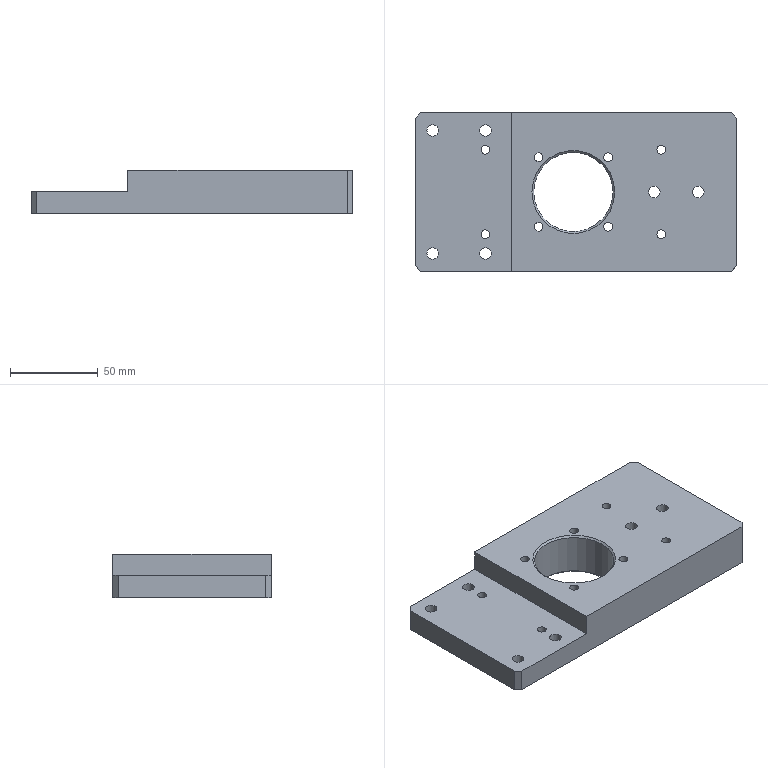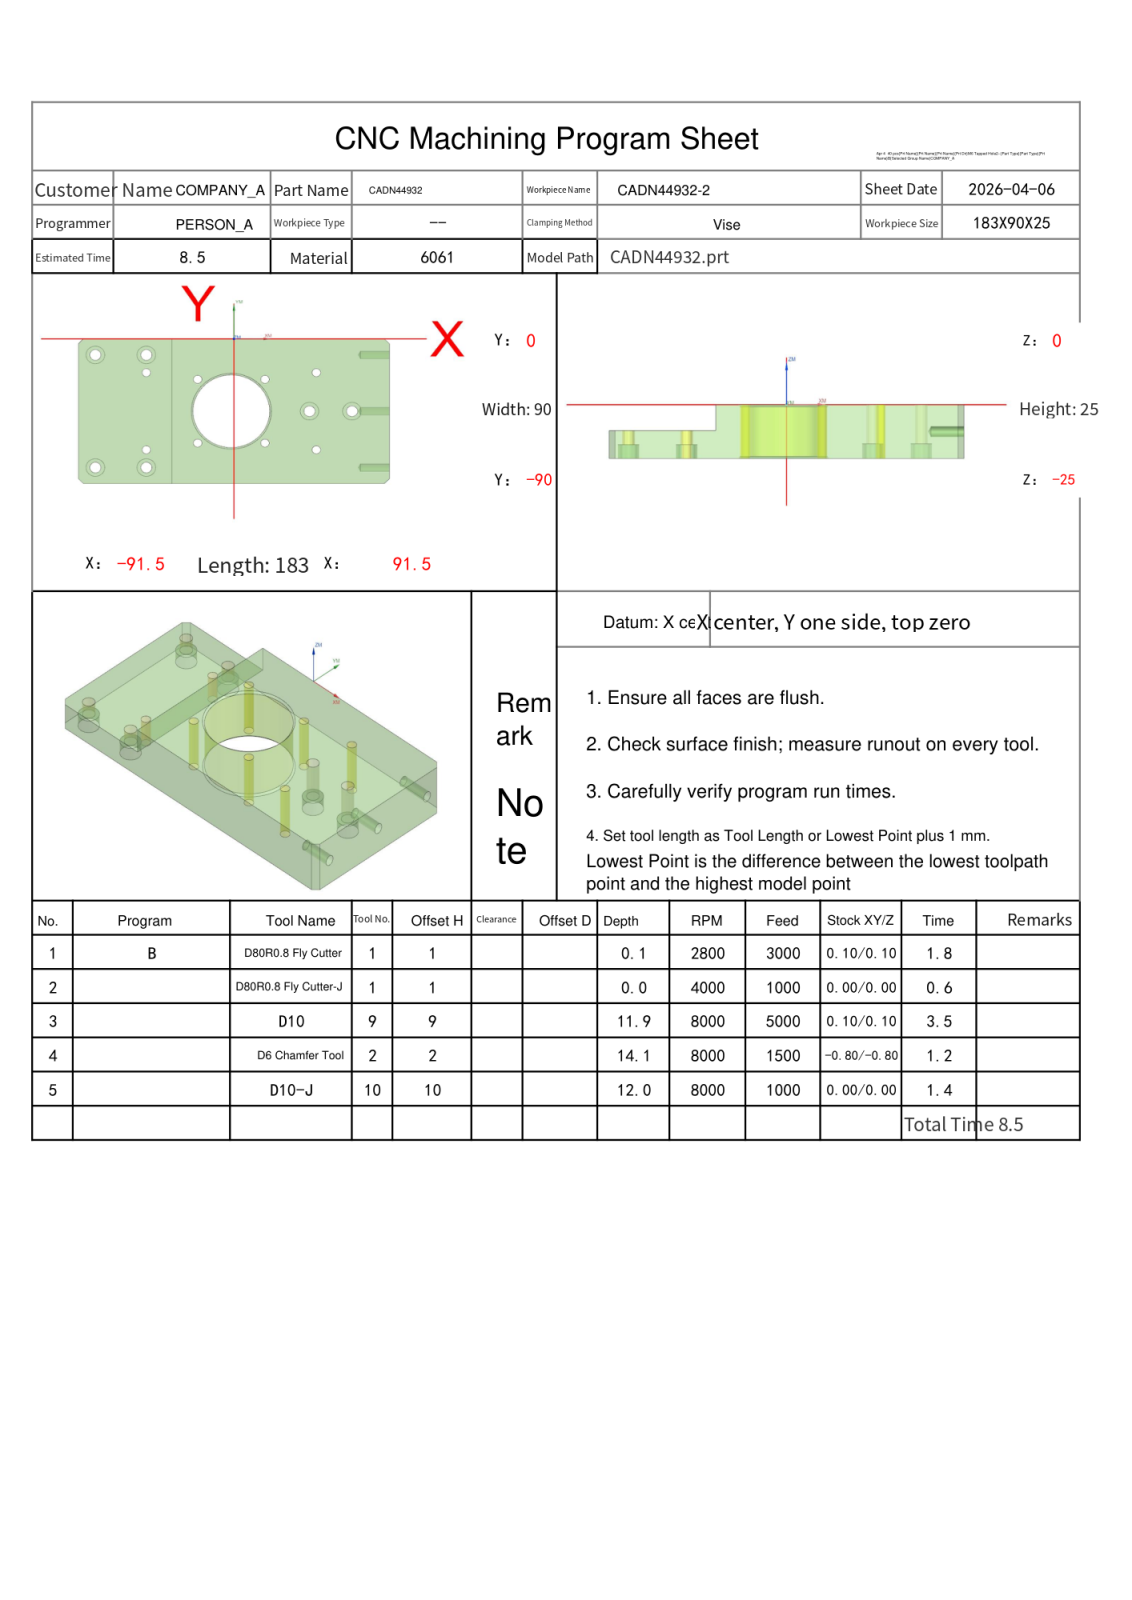NC program | NX | posted by the shop | part box 183 x 90 x 25 mm
Whole program:
%
O0001
(Machine time: 9.36 MIN)
(===Total Tool:4===)
(T1=D80R0.8 Fly Cutter D=80.  R=0.8  D-  H01 Z=0.    )
(T9=D10     D=10.  R=0.   D-  H09 Z=-11.9 )
(T2=D6 Chamfer Tool   D=6.   R=0.   D-  H02 Z=-14.1 )
(T10=D10-J  D=10.  R=0.   D10 H10 Z=-12.  )
G80 G90 G17 G49 G40
G91 G28 Z0
M01
N1 T01 M06
(D80R0.8 Fly Cutter  D=80. R=0.8 H=01 ce=0.10 di=0.10)
G00 G90 G54 X-143.597 Y-23.903 M03 S2800
G43 H01 Z20.
M08
Z6.011
G01 Z4.011 F3000.
X-131.597
X124.397
G02 X131.597 Y-31.103 I0.0 J-7.2
G01 Y-50.737
G02 X123.597 Y-58.737 I-8. J0.0
G01 X-131.597
X-143.597
Z6.011
G00 Y-23.903
Z5.522
G01 Z3.522
X-131.597
X124.397
G02 X131.597 Y-31.103 I0.0 J-7.2
G01 Y-50.737
G02 X123.597 Y-58.737 I-8. J0.0
G01 X-131.597
X-143.597
Z5.522
G00 Y-23.903
Z5.033
G01 Z3.033
X-131.597
X124.397
G02 X131.597 Y-31.103 I0.0 J-7.2
G01 Y-50.737
G02 X123.597 Y-58.737 I-8. J0.0
G01 X-131.597
X-143.597
Z5.033
G00 Y-23.903
Z4.544
G01 Z2.544
X-131.597
X124.397
G02 X131.597 Y-31.103 I0.0 J-7.2
G01 Y-50.737
G02 X123.597 Y-58.737 I-8. J0.0
G01 X-131.597
X-143.597
Z4.544
G00 Y-23.903
Z4.056
G01 Z2.056
X-131.597
X124.397
G02 X131.597 Y-31.103 I0.0 J-7.2
G01 Y-50.737
G02 X123.597 Y-58.737 I-8. J0.0
G01 X-131.597
X-143.597
Z4.056
G00 Y-23.903
Z3.567
G01 Z1.567
X-131.597
X124.397
G02 X131.597 Y-31.103 I0.0 J-7.2
G01 Y-50.737
G02 X123.597 Y-58.737 I-8. J0.0
G01 X-131.597
X-143.597
Z3.567
G00 Y-23.903
Z3.078
G01 Z1.078
X-131.597
X124.397
G02 X131.597 Y-31.103 I0.0 J-7.2
G01 Y-50.737
G02 X123.597 Y-58.737 I-8. J0.0
G01 X-131.597
X-143.597
Z3.078
G00 Y-23.903
Z2.589
G01 Z.589
X-131.597
X124.397
G02 X131.597 Y-31.103 I0.0 J-7.2
G01 Y-50.737
G02 X123.597 Y-58.737 I-8. J0.0
G01 X-131.597
X-143.597
Z2.589
G00 Y-23.903
Z2.1
G01 Z.1
X-131.597
X124.397
G02 X131.597 Y-31.103 I0.0 J-7.2
G01 Y-50.737
G02 X123.597 Y-58.737 I-8. J0.0
G01 X-131.597
X-143.597
Z2.1
G00 Z20.
G91 G28 Z0.0
M05
M09
G91 G28 Z0.0
M01
N2 T01 M06
(D80R0.8 Fly Cutter-J  D=80. R=0.8 H=01 ce=0.00 di=0.00)
G00 G90 G54 X-143.499 Y-24.001 M03 S4000
G43 H01 Z20.
M08
Z2.
G01 Z0.0 F1000.
X-131.499
X124.299
G02 X131.499 Y-31.201 I0.0 J-7.2
G01 Y-50.639
G02 X123.499 Y-58.639 I-8. J0.0
G01 X-131.499
X-143.499
Z2.
G00 Z20.
G91 G28 Z0.0
M05
M09
G91 G28 Z0.0
M01
N3 T09 M06
(D10  D=10. R=0. H=09 ce=0.10 di=0.10)
G00 G90 G54 X-94.1 Y5.714 M03 S8000
G43 H09 Z14.5
M08
Z.905
G01 Z-.595 F5000.
Y1.33
Y-90.916
G03 X-93.808 Y-91.622 I1. J.001
G01 X-90.822 Y-94.607
G03 X-90.116 Y-94.9 I.707 J.707
G01 X-87.599
G03 X-86.6 Y-93.901 I-.001 J1.
G01 Y3.901
G02 X-85.601 Y4.9 I1. J-.001
G01 X-80.099
G02 X-79.1 Y3.901 I-.001 J-1.
G01 Y-93.901
G03 X-78.101 Y-94.9 I1. J.001
G01 X-72.599
G03 X-71.6 Y-93.901 I-.001 J1.
G01 Y3.901
G02 X-70.601 Y4.9 I1. J-.001
G01 X-65.099
G02 X-64.1 Y3.901 I-.001 J-1.
G01 Y-93.901
G03 X-63.101 Y-94.9 I1. J.001
G01 X-57.599
G03 X-56.6 Y-93.901 I-.001 J1.
G01 Y3.901
G02 X-55.601 Y4.9 I1. J-.001
G01 X-50.099
G02 X-49.1 Y3.901 I-.001 J-1.
G01 Y-94.044
G03 X-48.255 Y-95.032 I1. J.001
G01 X-42.754 Y-95.888
X-42.6 Y-95.9
G03 X-41.6 Y-94.9 I0.0 J1.
G01 Y4.9
Y8.1
Z.905
G00 X-94.1 Y5.714
Z.31
G01 Z-1.19
Y1.33
Y-90.916
G03 X-93.808 Y-91.622 I1. J.001
G01 X-90.822 Y-94.607
G03 X-90.116 Y-94.9 I.707 J.707
G01 X-87.599
G03 X-86.6 Y-93.901 I-.001 J1.
G01 Y3.901
G02 X-85.601 Y4.9 I1. J-.001
G01 X-80.099
G02 X-79.1 Y3.901 I-.001 J-1.
G01 Y-93.901
G03 X-78.101 Y-94.9 I1. J.001
G01 X-72.599
G03 X-71.6 Y-93.901 I-.001 J1.
G01 Y3.901
G02 X-70.601 Y4.9 I1. J-.001
G01 X-65.099
G02 X-64.1 Y3.901 I-.001 J-1.
G01 Y-93.901
G03 X-63.101 Y-94.9 I1. J.001
G01 X-57.599
G03 X-56.6 Y-93.901 I-.001 J1.
G01 Y3.901
G02 X-55.601 Y4.9 I1. J-.001
G01 X-50.099
G02 X-49.1 Y3.901 I-.001 J-1.
G01 Y-94.044
G03 X-48.255 Y-95.032 I1. J.001
G01 X-42.754 Y-95.888
X-42.6 Y-95.9
G03 X-41.6 Y-94.9 I0.0 J1.
G01 Y4.9
Y8.1
Z.31
G00 X-94.1 Y5.714
Z-.285
G01 Z-1.785
Y1.33
Y-90.916
G03 X-93.808 Y-91.622 I1. J.001
G01 X-90.822 Y-94.607
G03 X-90.116 Y-94.9 I.707 J.707
G01 X-87.599
G03 X-86.6 Y-93.901 I-.001 J1.
G01 Y3.901
G02 X-85.601 Y4.9 I1. J-.001
G01 X-80.099
G02 X-79.1 Y3.901 I-.001 J-1.
G01 Y-93.901
G03 X-78.101 Y-94.9 I1. J.001
G01 X-72.599
G03 X-71.6 Y-93.901 I-.001 J1.
G01 Y3.901
G02 X-70.601 Y4.9 I1. J-.001
G01 X-65.099
G02 X-64.1 Y3.901 I-.001 J-1.
G01 Y-93.901
G03 X-63.101 Y-94.9 I1. J.001
G01 X-57.599
G03 X-56.6 Y-93.901 I-.001 J1.
G01 Y3.901
G02 X-55.601 Y4.9 I1. J-.001
G01 X-50.099
G02 X-49.1 Y3.901 I-.001 J-1.
G01 Y-94.044
G03 X-48.255 Y-95.032 I1. J.001
G01 X-42.754 Y-95.888
X-42.6 Y-95.9
G03 X-41.6 Y-94.9 I0.0 J1.
G01 Y4.9
Y8.1
Z-.285
G00 X-94.1 Y5.714
Z-.88
G01 Z-2.38
Y1.33
Y-90.916
G03 X-93.808 Y-91.622 I1. J.001
G01 X-90.822 Y-94.607
G03 X-90.116 Y-94.9 I.707 J.707
G01 X-87.599
G03 X-86.6 Y-93.901 I-.001 J1.
G01 Y3.901
G02 X-85.601 Y4.9 I1. J-.001
G01 X-80.099
G02 X-79.1 Y3.901 I-.001 J-1.
G01 Y-93.901
G03 X-78.101 Y-94.9 I1. J.001
G01 X-72.599
G03 X-71.6 Y-93.901 I-.001 J1.
G01 Y3.901
G02 X-70.601 Y4.9 I1. J-.001
G01 X-65.099
G02 X-64.1 Y3.901 I-.001 J-1.
G01 Y-93.901
G03 X-63.101 Y-94.9 I1. J.001
G01 X-57.599
G03 X-56.6 Y-93.901 I-.001 J1.
G01 Y3.901
G02 X-55.601 Y4.9 I1. J-.001
G01 X-50.099
G02 X-49.1 Y3.901 I-.001 J-1.
G01 Y-94.044
G03 X-48.255 Y-95.032 I1. J.001
G01 X-42.754 Y-95.888
X-42.6 Y-95.9
G03 X-41.6 Y-94.9 I0.0 J1.
G01 Y4.9
Y8.1
Z-.88
G00 X-94.1 Y5.714
Z-1.475
G01 Z-2.975
Y1.33
Y-90.916
G03 X-93.808 Y-91.622 I1. J.001
G01 X-90.822 Y-94.607
G03 X-90.116 Y-94.9 I.707 J.707
G01 X-87.599
G03 X-86.6 Y-93.901 I-.001 J1.
G01 Y3.901
G02 X-85.601 Y4.9 I1. J-.001
G01 X-80.099
G02 X-79.1 Y3.901 I-.001 J-1.
G01 Y-93.901
G03 X-78.101 Y-94.9 I1. J.001
G01 X-72.599
G03 X-71.6 Y-93.901 I-.001 J1.
G01 Y3.901
G02 X-70.601 Y4.9 I1. J-.001
G01 X-65.099
G02 X-64.1 Y3.901 I-.001 J-1.
G01 Y-93.901
G03 X-63.101 Y-94.9 I1. J.001
G01 X-57.599
G03 X-56.6 Y-93.901 I-.001 J1.
G01 Y3.901
G02 X-55.601 Y4.9 I1. J-.001
G01 X-50.099
G02 X-49.1 Y3.901 I-.001 J-1.
G01 Y-94.044
G03 X-48.255 Y-95.032 I1. J.001
G01 X-42.754 Y-95.888
X-42.6 Y-95.9
G03 X-41.6 Y-94.9 I0.0 J1.
G01 Y4.9
Y8.1
Z-1.475
G00 X-94.1 Y5.714
Z-2.07
G01 Z-3.57
Y1.33
Y-90.916
G03 X-93.808 Y-91.622 I1. J.001
G01 X-90.822 Y-94.607
G03 X-90.116 Y-94.9 I.707 J.707
G01 X-87.599
G03 X-86.6 Y-93.901 I-.001 J1.
G01 Y3.901
G02 X-85.601 Y4.9 I1. J-.001
G01 X-80.099
G02 X-79.1 Y3.901 I-.001 J-1.
G01 Y-93.901
G03 X-78.101 Y-94.9 I1. J.001
G01 X-72.599
G03 X-71.6 Y-93.901 I-.001 J1.
G01 Y3.901
G02 X-70.601 Y4.9 I1. J-.001
G01 X-65.099
G02 X-64.1 Y3.901 I-.001 J-1.
G01 Y-93.901
G03 X-63.101 Y-94.9 I1. J.001
G01 X-57.599
G03 X-56.6 Y-93.901 I-.001 J1.
G01 Y3.901
G02 X-55.601 Y4.9 I1. J-.001
G01 X-50.099
G02 X-49.1 Y3.901 I-.001 J-1.
G01 Y-94.044
G03 X-48.255 Y-95.032 I1. J.001
G01 X-42.754 Y-95.888
X-42.6 Y-95.9
G03 X-41.6 Y-94.9 I0.0 J1.
G01 Y4.9
Y8.1
Z-2.07
G00 X-94.1 Y5.714
Z-2.665
G01 Z-4.165
Y1.33
Y-90.916
G03 X-93.808 Y-91.622 I1. J.001
G01 X-90.822 Y-94.607
G03 X-90.116 Y-94.9 I.707 J.707
G01 X-87.599
G03 X-86.6 Y-93.901 I-.001 J1.
G01 Y3.901
G02 X-85.601 Y4.9 I1. J-.001
G01 X-80.099
G02 X-79.1 Y3.901 I-.001 J-1.
G01 Y-93.901
G03 X-78.101 Y-94.9 I1. J.001
G01 X-72.599
G03 X-71.6 Y-93.901 I-.001 J1.
G01 Y3.901
G02 X-70.601 Y4.9 I1. J-.001
G01 X-65.099
G02 X-64.1 Y3.901 I-.001 J-1.
G01 Y-93.901
G03 X-63.101 Y-94.9 I1. J.001
G01 X-57.599
G03 X-56.6 Y-93.901 I-.001 J1.
G01 Y3.901
G02 X-55.601 Y4.9 I1. J-.001
G01 X-50.099
G02 X-49.1 Y3.901 I-.001 J-1.
G01 Y-94.044
G03 X-48.255 Y-95.032 I1. J.001
G01 X-42.754 Y-95.888
X-42.6 Y-95.9
G03 X-41.6 Y-94.9 I0.0 J1.
G01 Y4.9
Y8.1
Z-2.665
G00 X-94.1 Y5.714
Z-3.26
G01 Z-4.76
Y1.33
Y-90.916
G03 X-93.808 Y-91.622 I1. J.001
G01 X-90.822 Y-94.607
G03 X-90.116 Y-94.9 I.707 J.707
G01 X-87.599
G03 X-86.6 Y-93.901 I-.001 J1.
G01 Y3.901
G02 X-85.601 Y4.9 I1. J-.001
G01 X-80.099
G02 X-79.1 Y3.901 I-.001 J-1.
G01 Y-93.901
G03 X-78.101 Y-94.9 I1. J.001
G01 X-72.599
G03 X-71.6 Y-93.901 I-.001 J1.
G01 Y3.901
G02 X-70.601 Y4.9 I1. J-.001
G01 X-65.099
G02 X-64.1 Y3.901 I-.001 J-1.
G01 Y-93.901
G03 X-63.101 Y-94.9 I1. J.001
G01 X-57.599
G03 X-56.6 Y-93.901 I-.001 J1.
G01 Y3.901
G02 X-55.601 Y4.9 I1. J-.001
G01 X-50.099
G02 X-49.1 Y3.901 I-.001 J-1.
G01 Y-94.044
G03 X-48.255 Y-95.032 I1. J.001
G01 X-42.754 Y-95.888
X-42.6 Y-95.9
G03 X-41.6 Y-94.9 I0.0 J1.
G01 Y4.9
Y8.1
Z-3.26
G00 X-94.1 Y5.714
Z-3.855
G01 Z-5.355
Y1.33
Y-90.916
G03 X-93.808 Y-91.622 I1. J.001
G01 X-90.822 Y-94.607
G03 X-90.116 Y-94.9 I.707 J.707
G01 X-87.599
G03 X-86.6 Y-93.901 I-.001 J1.
G01 Y3.901
G02 X-85.601 Y4.9 I1. J-.001
G01 X-80.099
G02 X-79.1 Y3.901 I-.001 J-1.
G01 Y-93.901
G03 X-78.101 Y-94.9 I1. J.001
G01 X-72.599
G03 X-71.6 Y-93.901 I-.001 J1.
G01 Y3.901
G02 X-70.601 Y4.9 I1. J-.001
G01 X-65.099
G02 X-64.1 Y3.901 I-.001 J-1.
G01 Y-93.901
G03 X-63.101 Y-94.9 I1. J.001
G01 X-57.599
G03 X-56.6 Y-93.901 I-.001 J1.
G01 Y3.901
G02 X-55.601 Y4.9 I1. J-.001
G01 X-50.099
G02 X-49.1 Y3.901 I-.001 J-1.
G01 Y-94.044
G03 X-48.255 Y-95.032 I1. J.001
G01 X-42.754 Y-95.888
X-42.6 Y-95.9
G03 X-41.6 Y-94.9 I0.0 J1.
G01 Y4.9
Y8.1
Z-3.855
G00 X-94.1 Y5.714
Z-4.45
G01 Z-5.95
Y1.33
Y-90.916
G03 X-93.808 Y-91.622 I1. J.001
G01 X-90.822 Y-94.607
G03 X-90.116 Y-94.9 I.707 J.707
G01 X-87.599
G03 X-86.6 Y-93.901 I-.001 J1.
G01 Y3.901
G02 X-85.601 Y4.9 I1. J-.001
G01 X-80.099
G02 X-79.1 Y3.901 I-.001 J-1.
G01 Y-93.901
G03 X-78.101 Y-94.9 I1. J.001
G01 X-72.599
G03 X-71.6 Y-93.901 I-.001 J1.
G01 Y3.901
G02 X-70.601 Y4.9 I1. J-.001
G01 X-65.099
G02 X-64.1 Y3.901 I-.001 J-1.
G01 Y-93.901
G03 X-63.101 Y-94.9 I1. J.001
G01 X-57.599
G03 X-56.6 Y-93.901 I-.001 J1.
G01 Y3.901
G02 X-55.601 Y4.9 I1. J-.001
G01 X-50.099
G02 X-49.1 Y3.901 I-.001 J-1.
G01 Y-94.044
G03 X-48.255 Y-95.032 I1. J.001
G01 X-42.754 Y-95.888
X-42.6 Y-95.9
G03 X-41.6 Y-94.9 I0.0 J1.
G01 Y4.9
Y8.1
Z-4.45
G00 X-94.1 Y5.714
Z-5.045
G01 Z-6.545
Y1.33
Y-90.916
G03 X-93.808 Y-91.622 I1. J.001
G01 X-90.822 Y-94.607
G03 X-90.116 Y-94.9 I.707 J.707
G01 X-87.599
G03 X-86.6 Y-93.901 I-.001 J1.
G01 Y3.901
G02 X-85.601 Y4.9 I1. J-.001
G01 X-80.099
G02 X-79.1 Y3.901 I-.001 J-1.
G01 Y-93.901
G03 X-78.101 Y-94.9 I1. J.001
G01 X-72.599
G03 X-71.6 Y-93.901 I-.001 J1.
G01 Y3.901
G02 X-70.601 Y4.9 I1. J-.001
G01 X-65.099
G02 X-64.1 Y3.901 I-.001 J-1.
G01 Y-93.901
G03 X-63.101 Y-94.9 I1. J.001
G01 X-57.599
G03 X-56.6 Y-93.901 I-.001 J1.
G01 Y3.901
G02 X-55.601 Y4.9 I1. J-.001
G01 X-50.099
G02 X-49.1 Y3.901 I-.001 J-1.
G01 Y-94.044
G03 X-48.255 Y-95.032 I1. J.001
G01 X-42.754 Y-95.888
X-42.6 Y-95.9
G03 X-41.6 Y-94.9 I0.0 J1.
G01 Y4.9
Y8.1
Z-5.045
G00 X-94.1 Y5.714
Z-5.64
G01 Z-7.14
Y1.33
Y-90.916
G03 X-93.808 Y-91.622 I1. J.001
G01 X-90.822 Y-94.607
G03 X-90.116 Y-94.9 I.707 J.707
G01 X-87.599
G03 X-86.6 Y-93.901 I-.001 J1.
G01 Y3.901
G02 X-85.601 Y4.9 I1. J-.001
G01 X-80.099
G02 X-79.1 Y3.901 I-.001 J-1.
G01 Y-93.901
G03 X-78.101 Y-94.9 I1. J.001
G01 X-72.599
G03 X-71.6 Y-93.901 I-.001 J1.
G01 Y3.901
G02 X-70.601 Y4.9 I1. J-.001
G01 X-65.099
G02 X-64.1 Y3.901 I-.001 J-1.
G01 Y-93.901
G03 X-63.101 Y-94.9 I1. J.001
G01 X-57.599
G03 X-56.6 Y-93.901 I-.001 J1.
G01 Y3.901
G02 X-55.601 Y4.9 I1. J-.001
G01 X-50.099
G02 X-49.1 Y3.901 I-.001 J-1.
G01 Y-94.044
G03 X-48.255 Y-95.032 I1. J.001
G01 X-42.754 Y-95.888
X-42.6 Y-95.9
G03 X-41.6 Y-94.9 I0.0 J1.
G01 Y4.9
Y8.1
Z-5.64
G00 X-94.1 Y5.714
Z-6.235
G01 Z-7.735
Y1.33
Y-90.916
G03 X-93.808 Y-91.622 I1. J.001
G01 X-90.822 Y-94.607
G03 X-90.116 Y-94.9 I.707 J.707
G01 X-87.599
G03 X-86.6 Y-93.901 I-.001 J1.
G01 Y3.901
G02 X-85.601 Y4.9 I1. J-.001
G01 X-80.099
G02 X-79.1 Y3.901 I-.001 J-1.
G01 Y-93.901
G03 X-78.101 Y-94.9 I1. J.001
G01 X-72.599
G03 X-71.6 Y-93.901 I-.001 J1.
G01 Y3.901
G02 X-70.601 Y4.9 I1. J-.001
G01 X-65.099
G02 X-64.1 Y3.901 I-.001 J-1.
G01 Y-93.901
G03 X-63.101 Y-94.9 I1. J.001
G01 X-57.599
G03 X-56.6 Y-93.901 I-.001 J1.
G01 Y3.901
G02 X-55.601 Y4.9 I1. J-.001
G01 X-50.099
G02 X-49.1 Y3.901 I-.001 J-1.
G01 Y-94.044
G03 X-48.255 Y-95.032 I1. J.001
G01 X-42.754 Y-95.888
X-42.6 Y-95.9
G03 X-41.6 Y-94.9 I0.0 J1.
G01 Y4.9
Y8.1
Z-6.235
G00 X-94.1 Y5.714
Z-6.83
G01 Z-8.33
Y1.33
Y-90.916
G03 X-93.808 Y-91.622 I1. J.001
G01 X-90.822 Y-94.607
G03 X-90.116 Y-94.9 I.707 J.707
G01 X-87.599
G03 X-86.6 Y-93.901 I-.001 J1.
G01 Y3.901
G02 X-85.601 Y4.9 I1. J-.001
G01 X-80.099
G02 X-79.1 Y3.901 I-.001 J-1.
G01 Y-93.901
G03 X-78.101 Y-94.9 I1. J.001
G01 X-72.599
G03 X-71.6 Y-93.901 I-.001 J1.
G01 Y3.901
G02 X-70.601 Y4.9 I1. J-.001
G01 X-65.099
G02 X-64.1 Y3.901 I-.001 J-1.
G01 Y-93.901
G03 X-63.101 Y-94.9 I1. J.001
G01 X-57.599
G03 X-56.6 Y-93.901 I-.001 J1.
G01 Y3.901
G02 X-55.601 Y4.9 I1. J-.001
G01 X-50.099
G02 X-49.1 Y3.901 I-.001 J-1.
G01 Y-94.044
G03 X-48.255 Y-95.032 I1. J.001
G01 X-42.754 Y-95.888
X-42.6 Y-95.9
G03 X-41.6 Y-94.9 I0.0 J1.
G01 Y4.9
Y8.1
Z-6.83
G00 X-94.1 Y5.714
Z-7.425
G01 Z-8.925
Y1.33
Y-90.916
G03 X-93.808 Y-91.622 I1. J.001
G01 X-90.822 Y-94.607
G03 X-90.116 Y-94.9 I.707 J.707
G01 X-87.599
G03 X-86.6 Y-93.901 I-.001 J1.
G01 Y3.901
G02 X-85.601 Y4.9 I1. J-.001
G01 X-80.099
G02 X-79.1 Y3.901 I-.001 J-1.
G01 Y-93.901
G03 X-78.101 Y-94.9 I1. J.001
G01 X-72.599
G03 X-71.6 Y-93.901 I-.001 J1.
G01 Y3.901
G02 X-70.601 Y4.9 I1. J-.001
G01 X-65.099
G02 X-64.1 Y3.901 I-.001 J-1.
G01 Y-93.901
G03 X-63.101 Y-94.9 I1. J.001
G01 X-57.599
G03 X-56.6 Y-93.901 I-.001 J1.
G01 Y3.901
G02 X-55.601 Y4.9 I1. J-.001
G01 X-50.099
G02 X-49.1 Y3.901 I-.001 J-1.
G01 Y-94.044
G03 X-48.255 Y-95.032 I1. J.001
G01 X-42.754 Y-95.888
X-42.6 Y-95.9
G03 X-41.6 Y-94.9 I0.0 J1.
G01 Y4.9
Y8.1
Z-7.425
G00 X-94.1 Y5.714
Z-8.02
G01 Z-9.52
Y1.33
Y-90.916
G03 X-93.808 Y-91.622 I1. J.001
G01 X-90.822 Y-94.607
G03 X-90.116 Y-94.9 I.707 J.707
G01 X-87.599
G03 X-86.6 Y-93.901 I-.001 J1.
G01 Y3.901
G02 X-85.601 Y4.9 I1. J-.001
G01 X-80.099
G02 X-79.1 Y3.901 I-.001 J-1.
G01 Y-93.901
G03 X-78.101 Y-94.9 I1. J.001
G01 X-72.599
G03 X-71.6 Y-93.901 I-.001 J1.
G01 Y3.901
G02 X-70.601 Y4.9 I1. J-.001
G01 X-65.099
G02 X-64.1 Y3.901 I-.001 J-1.
G01 Y-93.901
G03 X-63.101 Y-94.9 I1. J.001
G01 X-57.599
G03 X-56.6 Y-93.901 I-.001 J1.
G01 Y3.901
G02 X-55.601 Y4.9 I1. J-.001
G01 X-50.099
G02 X-49.1 Y3.901 I-.001 J-1.
G01 Y-94.044
G03 X-48.255 Y-95.032 I1. J.001
G01 X-42.754 Y-95.888
X-42.6 Y-95.9
G03 X-41.6 Y-94.9 I0.0 J1.
G01 Y4.9
Y8.1
Z-8.02
G00 X-94.1 Y5.714
Z-8.615
G01 Z-10.115
Y1.33
Y-90.916
G03 X-93.808 Y-91.622 I1. J.001
G01 X-90.822 Y-94.607
G03 X-90.116 Y-94.9 I.707 J.707
G01 X-87.599
G03 X-86.6 Y-93.901 I-.001 J1.
G01 Y3.901
G02 X-85.601 Y4.9 I1. J-.001
G01 X-80.099
G02 X-79.1 Y3.901 I-.001 J-1.
G01 Y-93.901
G03 X-78.101 Y-94.9 I1. J.001
G01 X-72.599
G03 X-71.6 Y-93.901 I-.001 J1.
G01 Y3.901
G02 X-70.601 Y4.9 I1. J-.001
G01 X-65.099
G02 X-64.1 Y3.901 I-.001 J-1.
G01 Y-93.901
G03 X-63.101 Y-94.9 I1. J.001
G01 X-57.599
G03 X-56.6 Y-93.901 I-.001 J1.
G01 Y3.901
G02 X-55.601 Y4.9 I1. J-.001
G01 X-50.099
G02 X-49.1 Y3.901 I-.001 J-1.
G01 Y-94.044
G03 X-48.255 Y-95.032 I1. J.001
G01 X-42.754 Y-95.888
X-42.6 Y-95.9
G03 X-41.6 Y-94.9 I0.0 J1.
G01 Y4.9
Y8.1
Z-8.615
G00 X-94.1 Y5.714
Z-9.21
G01 Z-10.71
Y1.33
Y-90.916
G03 X-93.808 Y-91.622 I1. J.001
G01 X-90.822 Y-94.607
G03 X-90.116 Y-94.9 I.707 J.707
G01 X-87.599
G03 X-86.6 Y-93.901 I-.001 J1.
G01 Y3.901
G02 X-85.601 Y4.9 I1. J-.001
G01 X-80.099
G02 X-79.1 Y3.901 I-.001 J-1.
G01 Y-93.901
G03 X-78.101 Y-94.9 I1. J.001
G01 X-72.599
G03 X-71.6 Y-93.901 I-.001 J1.
G01 Y3.901
G02 X-70.601 Y4.9 I1. J-.001
G01 X-65.099
G02 X-64.1 Y3.901 I-.001 J-1.
G01 Y-93.901
G03 X-63.101 Y-94.9 I1. J.001
G01 X-57.599
G03 X-56.6 Y-93.901 I-.001 J1.
G01 Y3.901
G02 X-55.601 Y4.9 I1. J-.001
G01 X-50.099
G02 X-49.1 Y3.901 I-.001 J-1.
G01 Y-94.044
G03 X-48.255 Y-95.032 I1. J.001
G01 X-42.754 Y-95.888
X-42.6 Y-95.9
G03 X-41.6 Y-94.9 I0.0 J1.
G01 Y4.9
Y8.1
Z-9.21
G00 X-94.1 Y5.714
Z-9.805
G01 Z-11.305
Y1.33
Y-90.916
G03 X-93.808 Y-91.622 I1. J.001
G01 X-90.822 Y-94.607
G03 X-90.116 Y-94.9 I.707 J.707
G01 X-87.599
G03 X-86.6 Y-93.901 I-.001 J1.
G01 Y3.901
G02 X-85.601 Y4.9 I1. J-.001
G01 X-80.099
G02 X-79.1 Y3.901 I-.001 J-1.
G01 Y-93.901
G03 X-78.101 Y-94.9 I1. J.001
G01 X-72.599
G03 X-71.6 Y-93.901 I-.001 J1.
G01 Y3.901
G02 X-70.601 Y4.9 I1. J-.001
G01 X-65.099
G02 X-64.1 Y3.901 I-.001 J-1.
G01 Y-93.901
G03 X-63.101 Y-94.9 I1. J.001
G01 X-57.599
G03 X-56.6 Y-93.901 I-.001 J1.
G01 Y3.901
G02 X-55.601 Y4.9 I1. J-.001
G01 X-50.099
G02 X-49.1 Y3.901 I-.001 J-1.
G01 Y-94.044
G03 X-48.255 Y-95.032 I1. J.001
G01 X-42.754 Y-95.888
X-42.6 Y-95.9
G03 X-41.6 Y-94.9 I0.0 J1.
G01 Y4.9
Y8.1
Z-9.805
G00 X-94.1 Y5.714
Z-10.4
G01 Z-11.9
Y1.33
Y-90.916
G03 X-93.808 Y-91.622 I1. J.001
G01 X-90.822 Y-94.607
G03 X-90.116 Y-94.9 I.707 J.707
G01 X-87.599
G03 X-86.6 Y-93.901 I-.001 J1.
G01 Y3.901
G02 X-85.601 Y4.9 I1. J-.001
G01 X-80.099
G02 X-79.1 Y3.901 I-.001 J-1.
G01 Y-93.901
G03 X-78.101 Y-94.9 I1. J.001
G01 X-72.599
G03 X-71.6 Y-93.901 I-.001 J1.
G01 Y3.901
G02 X-70.601 Y4.9 I1. J-.001
G01 X-65.099
G02 X-64.1 Y3.901 I-.001 J-1.
G01 Y-93.901
G03 X-63.101 Y-94.9 I1. J.001
G01 X-57.599
G03 X-56.6 Y-93.901 I-.001 J1.
G01 Y3.901
G02 X-55.601 Y4.9 I1. J-.001
G01 X-50.099
G02 X-49.1 Y3.901 I-.001 J-1.
G01 Y-94.044
G03 X-48.255 Y-95.032 I1. J.001
G01 X-42.754 Y-95.888
X-42.6 Y-95.9
G03 X-41.6 Y-94.9 I0.0 J1.
G01 Y4.9
Y8.1
Z-10.4
G00 Z14.5
G91 G28 Z0.0
M05
M09
G91 G28 Z0.0
M01
N4 T02 M06
(D6 Chamfer Tool  D=6. R=0. H=02 ce=-0.30 di=0.00)
G00 G90 G54 X18.27 Y-54.309 M03 S7000
G43 H02 Z20.
M08
Z2.5
G01 X18.288 Y-54.272 Z2.485 F1500.
X18.701 Y-53.335 Z2.112
X19.069 Y-52.38 Z1.74
X19.392 Y-51.409 Z1.367
X19.669 Y-50.424 Z.995
X19.9 Y-49.426 Z.622
X20.084 Y-48.419 Z.25
X20.22 Y-47.405 Z-.123
X20.309 Y-46.385 Z-.496
X20.35 Y-45.362 Z-.868
Y-45. Z-1.
G03 X-1.5 Y-23.15 I-21.85 J0.0
X-23.35 Y-45. I0.0 J-21.85
X-1.5 Y-66.85 I21.85 J0.0
X20.35 Y-45. I0.0 J21.85
X20.344 Y-44.5 I-21.85 J0.0
G01 Z1.5
G00 Z20.
G00 G90 X48.732 Y-21.87 M03 S8000
Z20.
Z-.9
G01 Z-1.4 F600.
X48.9 Y-22.5
G03 X50.4 Y-21. I0.0 J1.5
X48.5 Y-19.1 I-1.9 J0.0
X46.6 Y-21. I0.0 J-1.9
X48.5 Y-22.9 I1.9 J0.0
X50.4 Y-21. I0.0 J1.9
X48.9 Y-19.5 I-1.5 J0.0
G01 X48.732 Y-20.13
Z-.9
G00 Z20.
X18.531 Y-26.071
Z-.9
G01 Z-1.4
X18.699 Y-26.701
G03 X20.199 Y-25.201 I0.0 J1.5
X18.299 Y-23.301 I-1.9 J0.0
X16.399 Y-25.201 I0.0 J-1.9
X18.299 Y-27.101 I1.9 J0.0
X20.199 Y-25.201 I0.0 J1.9
X18.699 Y-23.701 I-1.5 J0.0
G01 X18.531 Y-24.331
Z-.9
G00 Z20.
X-21.067 Y-26.071
Z-.9
G01 Z-1.4
X-20.899 Y-26.701
G03 X-19.399 Y-25.201 I0.0 J1.5
X-21.299 Y-23.301 I-1.9 J0.0
X-23.199 Y-25.201 I0.0 J-1.9
X-21.299 Y-27.101 I1.9 J0.0
X-19.399 Y-25.201 I0.0 J1.9
X-20.899 Y-23.701 I-1.5 J0.0
G01 X-21.067 Y-24.331
Z-.9
G00 Z20.
Y-65.669
Z-.9
G01 Z-1.4
X-20.899 Y-66.299
G03 X-19.399 Y-64.799 I0.0 J1.5
X-21.299 Y-62.899 I-1.9 J0.0
X-23.199 Y-64.799 I0.0 J-1.9
X-21.299 Y-66.699 I1.9 J0.0
X-19.399 Y-64.799 I0.0 J1.9
X-20.899 Y-63.299 I-1.5 J0.0
G01 X-21.067 Y-63.929
Z-.9
G00 Z20.
X18.531 Y-65.669
Z-.9
G01 Z-1.4
X18.699 Y-66.299
G03 X20.199 Y-64.799 I0.0 J1.5
X18.299 Y-62.899 I-1.9 J0.0
X16.399 Y-64.799 I0.0 J-1.9
X18.299 Y-66.699 I1.9 J0.0
X20.199 Y-64.799 I0.0 J1.9
X18.699 Y-63.299 I-1.5 J0.0
G01 X18.531 Y-63.929
Z-.9
G00 Z20.
X48.732 Y-69.87
Z-.9
G01 Z-1.4
X48.9 Y-70.5
G03 X50.4 Y-69. I0.0 J1.5
X48.5 Y-67.1 I-1.9 J0.0
X46.6 Y-69. I0.0 J-1.9
X48.5 Y-70.9 I1.9 J0.0
X50.4 Y-69. I0.0 J1.9
X48.9 Y-67.5 I-1.5 J0.0
G01 X48.732 Y-68.13
Z-.9
G00 Z20.
G00 G90 X-51.437 Y-69.19 M03 S8000
Z20.
Z-13.6
G01 Z-14.1 F600.
X-51.426 Y-69.224
G03 X-51.133 Y-69.253 I.293 J1.471
X-50.3 Y-69. I0.0 J1.5
X-51.5 Y-67.8 I-1.2 J0.0
X-52.7 Y-69. I0.0 J-1.2
X-51.5 Y-70.2 I1.2 J0.0
X-50.3 Y-69. I0.0 J1.2
X-51.133 Y-68.747 I-.833 J-1.247
X-51.426 Y-68.776 I0.0 J-1.5
G01 X-51.437 Y-68.81
Z-13.6
G00 Z20.
Y-21.19
Z-13.6
G01 Z-14.1
X-51.426 Y-21.224
G03 X-51.133 Y-21.253 I.293 J1.471
X-50.3 Y-21. I0.0 J1.5
X-51.5 Y-19.8 I-1.2 J0.0
X-52.7 Y-21. I0.0 J-1.2
X-51.5 Y-22.2 I1.2 J0.0
X-50.3 Y-21. I0.0 J1.2
X-51.133 Y-20.747 I-.833 J-1.247
X-51.426 Y-20.776 I0.0 J-1.5
G01 X-51.437 Y-20.81
Z-13.6
G00 Z20.
G00 G90 X25.614 Y1.227 M03 S6500
Z20.
Z.172
G01 Z-1.2 F1500.
G03 X25.9 Y1.027 I1.286 J1.532
G01 X25.946 Y.997
X26. Y1.
X88.5
X88.759 Y.966
X89. Y.866
X89.207 Y.707
X92.207 Y-2.293
X92.366 Y-2.5
X92.466 Y-2.741
X92.5 Y-3.
Y-87.
X92.466 Y-87.259
X92.366 Y-87.5
X92.207 Y-87.707
X89.207 Y-90.707
X89. Y-90.866
X88.759 Y-90.966
X88.5 Y-91.
X-36.5
G02 X-37.5 Y-90. I0.0 J1.
G01 Y0.0
G02 X-36.5 Y1. I1. J0.0
G01 X26.
X26.054 Y.997
X26.1 Y1.027
G03 X26.386 Y1.227 I-1. J1.732
G01 Z.172
G00 Z10.
X-19.984 Y-65.206
Z.284
G01 Z-1.2
G03 X-19.815 Y-64.901 I-1.658 J1.118
G01 X-19.79 Y-64.853
X-19.799 Y-64.799
G03 X-21.299 Y-63.299 I-1.5 J0.0
X-22.799 Y-64.799 I0.0 J-1.5
X-21.299 Y-66.299 I1.5 J0.0
X-19.799 Y-64.799 I0.0 J1.5
G01 X-19.79 Y-64.745
X-19.815 Y-64.697
G03 X-19.984 Y-64.392 I-1.827 J-.813
G01 Z.284
G00 Z10.
Y-25.608
Z.284
G01 Z-1.2
G03 X-19.815 Y-25.303 I-1.658 J1.118
G01 X-19.79 Y-25.255
X-19.799 Y-25.201
G03 X-21.299 Y-23.701 I-1.5 J0.0
X-22.799 Y-25.201 I0.0 J-1.5
X-21.299 Y-26.701 I1.5 J0.0
X-19.799 Y-25.201 I0.0 J1.5
G01 X-19.79 Y-25.147
X-19.815 Y-25.099
G03 X-19.984 Y-24.794 I-1.827 J-.813
G01 Z.284
G00 Z10.
X19.614 Y-25.608
Z.284
G01 Z-1.2
G03 X19.783 Y-25.303 I-1.658 J1.118
G01 X19.808 Y-25.255
X19.799 Y-25.201
G03 X18.299 Y-23.701 I-1.5 J0.0
X16.799 Y-25.201 I0.0 J-1.5
X18.299 Y-26.701 I1.5 J0.0
X19.799 Y-25.201 I0.0 J1.5
G01 X19.808 Y-25.147
X19.783 Y-25.099
G03 X19.614 Y-24.794 I-1.827 J-.813
G01 Z.284
G00 Z10.
X49.815 Y-21.407
Z.284
G01 Z-1.2
G03 X49.984 Y-21.102 I-1.658 J1.118
G01 X50.009 Y-21.054
X50. Y-21.
G03 X48.5 Y-19.5 I-1.5 J0.0
X47. Y-21. I0.0 J-1.5
X48.5 Y-22.5 I1.5 J0.0
X50. Y-21. I0.0 J1.5
G01 X50.009 Y-20.946
X49.984 Y-20.898
G03 X49.815 Y-20.593 I-1.827 J-.813
G01 Z.284
G00 Z10.
X71.608 Y-45.404
Z.253
G01 Z-1.2
G03 X71.782 Y-45.102 I-1.638 J1.147
G01 X71.808 Y-45.054
X71.8 Y-45.
G03 X69.5 Y-42.7 I-2.3 J0.0
X67.2 Y-45. I0.0 J-2.3
X69.5 Y-47.3 I2.3 J0.0
X71.8 Y-45. I0.0 J2.3
G01 X71.808 Y-44.946
X71.782 Y-44.898
G03 X71.608 Y-44.596 I-1.813 J-.845
G01 Z.253
G00 Z10.
X46.608 Y-45.404
Z.253
G01 Z-1.2
G03 X46.782 Y-45.102 I-1.638 J1.147
G01 X46.808 Y-45.054
X46.8 Y-45.
G03 X44.5 Y-42.7 I-2.3 J0.0
X42.2 Y-45. I0.0 J-2.3
X44.5 Y-47.3 I2.3 J0.0
X46.8 Y-45. I0.0 J2.3
G01 X46.808 Y-44.946
X46.782 Y-44.898
G03 X46.608 Y-44.596 I-1.813 J-.845
G01 Z.253
G00 Z10.
X49.815 Y-69.407
Z.284
G01 Z-1.2
G03 X49.984 Y-69.102 I-1.658 J1.118
G01 X50.009 Y-69.054
X50. Y-69.
G03 X48.5 Y-67.5 I-1.5 J0.0
X47. Y-69. I0.0 J-1.5
X48.5 Y-70.5 I1.5 J0.0
X50. Y-69. I0.0 J1.5
G01 X50.009 Y-68.946
X49.984 Y-68.898
G03 X49.815 Y-68.593 I-1.827 J-.813
G01 Z.284
G00 Z10.
X19.614 Y-65.206
Z.284
G01 Z-1.2
G03 X19.783 Y-64.901 I-1.658 J1.118
G01 X19.808 Y-64.853
X19.799 Y-64.799
G03 X18.299 Y-63.299 I-1.5 J0.0
X16.799 Y-64.799 I0.0 J-1.5
X18.299 Y-66.299 I1.5 J0.0
X19.799 Y-64.799 I0.0 J1.5
G01 X19.808 Y-64.745
X19.783 Y-64.697
G03 X19.614 Y-64.392 I-1.827 J-.813
G01 Z.284
G00 Z10.
X-39.507 Y-91.068
Z-1.793
G01 Z-13.2
X-39.593 Y-91.008
X-39.623 Y-91.
X-88.5
X-88.759 Y-90.966
X-89. Y-90.866
X-89.207 Y-90.707
X-92.207 Y-87.707
X-92.366 Y-87.5
X-92.466 Y-87.259
X-92.5 Y-87.
Y-3.
X-92.466 Y-2.741
X-92.366 Y-2.5
X-92.207 Y-2.293
X-89.207 Y.707
X-89. Y.866
X-88.759 Y.966
X-88.5 Y1.
X-39.623
X-39.593 Y1.008
X-39.507 Y1.068
Z-1.793
G00 Z10.
X-79.392 Y-10.404
Z-11.747
G01 Z-13.2
G03 X-79.218 Y-10.102 I-1.638 J1.147
G01 X-79.192 Y-10.054
X-79.2 Y-10.
G03 X-81.5 Y-7.7 I-2.3 J0.0
X-83.8 Y-10. I0.0 J-2.3
X-81.5 Y-12.3 I2.3 J0.0
X-79.2 Y-10. I0.0 J2.3
G01 X-79.192 Y-9.946
X-79.218 Y-9.898
G03 X-79.392 Y-9.596 I-1.813 J-.845
G01 Z-11.747
G00 Z10.
X-49.392 Y-10.404
Z-11.747
G01 Z-13.2
G03 X-49.218 Y-10.102 I-1.638 J1.147
G01 X-49.192 Y-10.054
X-49.2 Y-10.
G03 X-51.5 Y-7.7 I-2.3 J0.0
X-53.8 Y-10. I0.0 J-2.3
X-51.5 Y-12.3 I2.3 J0.0
X-49.2 Y-10. I0.0 J2.3
G01 X-49.192 Y-9.946
X-49.218 Y-9.898
G03 X-49.392 Y-9.596 I-1.813 J-.845
G01 Z-11.747
G00 Z-9.45
X-50.185 Y-21.407
Z-11.716
G01 Z-13.2
G03 X-50.016 Y-21.102 I-1.658 J1.118
G01 X-49.991 Y-21.054
X-50. Y-21.
G03 X-51.5 Y-19.5 I-1.5 J0.0
X-53. Y-21. I0.0 J-1.5
X-51.5 Y-22.5 I1.5 J0.0
X-50. Y-21. I0.0 J1.5
G01 X-49.991 Y-20.946
X-50.016 Y-20.898
G03 X-50.185 Y-20.593 I-1.827 J-.813
G01 Z-11.716
G00 Z10.
Y-69.407
Z-11.716
G01 Z-13.2
G03 X-50.016 Y-69.102 I-1.658 J1.118
G01 X-49.991 Y-69.054
X-50. Y-69.
G03 X-51.5 Y-67.5 I-1.5 J0.0
X-53. Y-69. I0.0 J-1.5
X-51.5 Y-70.5 I1.5 J0.0
X-50. Y-69. I0.0 J1.5
G01 X-49.991 Y-68.946
X-50.016 Y-68.898
G03 X-50.185 Y-68.593 I-1.827 J-.813
G01 Z-11.716
G00 Z-9.45
X-49.392 Y-80.404
Z-11.747
G01 Z-13.2
G03 X-49.218 Y-80.102 I-1.638 J1.147
G01 X-49.192 Y-80.054
X-49.2 Y-80.
G03 X-51.5 Y-77.7 I-2.3 J0.0
X-53.8 Y-80. I0.0 J-2.3
X-51.5 Y-82.3 I2.3 J0.0
X-49.2 Y-80. I0.0 J2.3
G01 X-49.192 Y-79.946
X-49.218 Y-79.898
G03 X-49.392 Y-79.596 I-1.813 J-.845
G01 Z-11.747
G00 Z10.
X-79.392 Y-80.404
Z-11.747
G01 Z-13.2
G03 X-79.218 Y-80.102 I-1.638 J1.147
G01 X-79.192 Y-80.054
X-79.2 Y-80.
G03 X-81.5 Y-77.7 I-2.3 J0.0
X-83.8 Y-80. I0.0 J-2.3
X-81.5 Y-82.3 I2.3 J0.0
X-79.2 Y-80. I0.0 J2.3
G01 X-79.192 Y-79.946
X-79.218 Y-79.898
G03 X-79.392 Y-79.596 I-1.813 J-.845
G01 Z-11.747
G00 Z20.
G00 G90 X-.3 Y-24.385 M03 S6500
Z20.
Z-.2
G01 Z-1.7 F1500.
Y-24.35
G03 X-1.5 Y-23.15 I-1.2 J0.0
X-23.35 Y-45. I0.0 J-21.85
X-1.5 Y-66.85 I21.85 J0.0
X20.35 Y-45. I0.0 J21.85
X-1.5 Y-23.15 I-21.85 J0.0
X-1.9 Y-23.154 I0.0 J-21.85
X-3.078 Y-24.353 I.022 J-1.2
G01 Y-24.375
X-3.077 Y-24.41
Z-.2
G00 Z20.
G91 G28 Z0.0
M05
M09
G91 G28 Z0.0
M01
N5 T10 M06
(D10-J  D=10. R=0. H=10 ce=0.40 di=0.00)
G00 G90 G54 X-93.562 Y-94.837 M03 S8000
G43 H10 Z14.5
M08
Z-10.5
G01 Z-12. F1000.
G03 X-92.5 Y-93.071 I-.938 J1.766
G01 Y2.658
G02 X-92.208 Y3.363 I1. J-.001
G01 X-90.864 Y4.707
G02 X-90.157 Y5. I.707 J-.707
G01 X-88.899
G02 X-87.9 Y4.001 I-.001 J-1.
G01 Y-94.1
G03 X-87. Y-95. I.9 J0.0
G01 X-84.3
G03 X-83.3 Y-94. I0.0 J1.
G01 Y4.1
G02 X-82.4 Y5. I.9 J0.0
G01 X-79.7
G02 X-78.7 Y4. I0.0 J-1.
G01 Y-94.1
G03 X-77.8 Y-95. I.9 J0.0
G01 X-75.1
G03 X-74.1 Y-94. I0.0 J1.
G01 Y4.1
G02 X-73.2 Y5. I.9 J0.0
G01 X-70.5
G02 X-69.5 Y4. I0.0 J-1.
G01 Y-94.1
G03 X-68.6 Y-95. I.9 J0.0
G01 X-65.9
G03 X-64.9 Y-94. I0.0 J1.
G01 Y4.1
G02 X-64. Y5. I.9 J0.0
G01 X-61.3
G02 X-60.3 Y4. I0.0 J-1.
G01 Y-94.1
G03 X-59.4 Y-95. I.9 J0.0
G01 X-56.7
G03 X-55.7 Y-94. I0.0 J1.
G01 Y4.1
G02 X-54.8 Y5. I.9 J0.0
G01 X-52.1
G02 X-51.1 Y4. I0.0 J-1.
G01 Y-94.1
G03 X-50.2 Y-95. I.9 J0.0
G01 X-47.5
G03 X-46.5 Y-94. I0.0 J1.
G01 Y4.1
G02 X-45.6 Y5. I.9 J0.0
G01 X-42.9
G02 X-41.9 Y4. I0.0 J-1.
G01 Y-95.
G02 X-43.9 Y-97. I-2. J0.0
G01 Z-10.5
G00 Z14.5
G00 G90 X-43.699 Y-97. M03 S8000
Z14.5
Z-11.
G01 Z-12. F1000.
G41 D10
X-43.499
G03 X-41.5 Y-95. I-.001 J2.
G01 Y5.
G03 X-43.499 Y7. I-2. J0.0
G01 G40 X-43.699
Z-11.
G00 Z14.5
M05
M09
G91 G28 Z0.0
G91 G28 Y0.0
M30
%